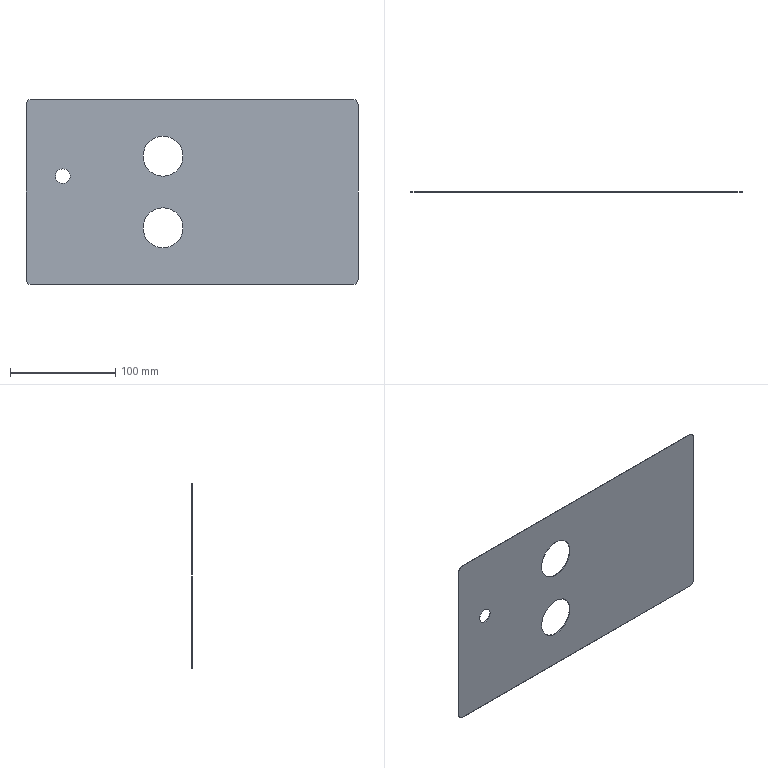Part | SolidWorks | features Extrusion 1 | 1 solid | 16 faces | box 315 x 0.6 x 176 mm | volume 31798 mm3 | cylinder 10 | plane 6 | commonest cylinder face diameters 10 x4 38 x4 14 x2
STEP:
#1=CARTESIAN_POINT('',(-95.,0.3,8.));
#2=VERTEX_POINT('',#1);
#3=CARTESIAN_POINT('',(-95.,0.3,22.));
#4=VERTEX_POINT('',#3);
#5=CARTESIAN_POINT('',(-95.,0.3,15.));
#6=DIRECTION('',(0.,1.,0.));
#7=DIRECTION('',(0.,0.,1.));
#8=AXIS2_PLACEMENT_3D('',#5,#6,#7);
#9=CIRCLE('',#8,7.);
#10=EDGE_CURVE('',#2,#4,#9,.T.);
#11=ORIENTED_EDGE('',*,*,#10,.T.);
#12=CARTESIAN_POINT('',(-95.,-0.3,22.));
#13=VERTEX_POINT('',#12);
#14=CARTESIAN_POINT('',(-95.,0.3,22.));
#15=DIRECTION('',(0.,-1.,0.));
#16=VECTOR('',#15,1000.);
#17=LINE('',#14,#16);
#18=EDGE_CURVE('',#4,#13,#17,.T.);
#19=ORIENTED_EDGE('',*,*,#18,.T.);
#20=CARTESIAN_POINT('',(-95.,-0.3,8.));
#21=VERTEX_POINT('',#20);
#22=CARTESIAN_POINT('',(-95.,-0.3,15.));
#23=DIRECTION('',(0.,1.,0.));
#24=DIRECTION('',(0.,0.,1.));
#25=AXIS2_PLACEMENT_3D('',#22,#23,#24);
#26=CIRCLE('',#25,7.);
#27=EDGE_CURVE('',#21,#13,#26,.T.);
#28=ORIENTED_EDGE('',*,*,#27,.F.);
#29=CARTESIAN_POINT('',(-95.,0.3,8.));
#30=DIRECTION('',(0.,-1.,0.));
#31=VECTOR('',#30,1000.);
#32=LINE('',#29,#31);
#33=EDGE_CURVE('',#2,#21,#32,.T.);
#34=ORIENTED_EDGE('',*,*,#33,.F.);
#35=EDGE_LOOP('',(#11,#19,#28,#34));
#36=FACE_OUTER_BOUND('',#35,.T.);
#37=CARTESIAN_POINT('',(-95.,0.3,15.));
#38=DIRECTION('',(0.,-1.,0.));
#39=DIRECTION('',(0.,0.,-1.));
#40=AXIS2_PLACEMENT_3D('',#37,#38,#39);
#41=CYLINDRICAL_SURFACE('',#40,7.);
#42=ADVANCED_FACE('',(#36),#41,.F.);
#43=CARTESIAN_POINT('',(0.,0.3,15.));
#44=VERTEX_POINT('',#43);
#45=CARTESIAN_POINT('',(0.,0.3,53.));
#46=VERTEX_POINT('',#45);
#47=CARTESIAN_POINT('',(0.,0.3,34.));
#48=DIRECTION('',(0.,1.,0.));
#49=DIRECTION('',(0.,0.,1.));
#50=AXIS2_PLACEMENT_3D('',#47,#48,#49);
#51=CIRCLE('',#50,19.);
#52=EDGE_CURVE('',#44,#46,#51,.T.);
#53=ORIENTED_EDGE('',*,*,#52,.T.);
#54=CARTESIAN_POINT('',(0.,-0.3,53.));
#55=VERTEX_POINT('',#54);
#56=CARTESIAN_POINT('',(0.,0.3,53.));
#57=DIRECTION('',(0.,-1.,0.));
#58=VECTOR('',#57,1000.);
#59=LINE('',#56,#58);
#60=EDGE_CURVE('',#46,#55,#59,.T.);
#61=ORIENTED_EDGE('',*,*,#60,.T.);
#62=CARTESIAN_POINT('',(0.,-0.3,15.));
#63=VERTEX_POINT('',#62);
#64=CARTESIAN_POINT('',(0.,-0.3,34.));
#65=DIRECTION('',(0.,1.,0.));
#66=DIRECTION('',(0.,0.,1.));
#67=AXIS2_PLACEMENT_3D('',#64,#65,#66);
#68=CIRCLE('',#67,19.);
#69=EDGE_CURVE('',#63,#55,#68,.T.);
#70=ORIENTED_EDGE('',*,*,#69,.F.);
#71=CARTESIAN_POINT('',(0.,0.3,15.));
#72=DIRECTION('',(0.,-1.,0.));
#73=VECTOR('',#72,1000.);
#74=LINE('',#71,#73);
#75=EDGE_CURVE('',#44,#63,#74,.T.);
#76=ORIENTED_EDGE('',*,*,#75,.F.);
#77=EDGE_LOOP('',(#53,#61,#70,#76));
#78=FACE_OUTER_BOUND('',#77,.T.);
#79=CARTESIAN_POINT('',(0.,0.3,34.));
#80=DIRECTION('',(0.,-1.,0.));
#81=DIRECTION('',(0.,0.,-1.));
#82=AXIS2_PLACEMENT_3D('',#79,#80,#81);
#83=CYLINDRICAL_SURFACE('',#82,19.);
#84=ADVANCED_FACE('',(#78),#83,.F.);
#85=CARTESIAN_POINT('',(0.,0.3,-53.));
#86=VERTEX_POINT('',#85);
#87=CARTESIAN_POINT('',(0.,0.3,-15.));
#88=VERTEX_POINT('',#87);
#89=CARTESIAN_POINT('',(0.,0.3,-34.));
#90=DIRECTION('',(0.,1.,0.));
#91=DIRECTION('',(0.,0.,1.));
#92=AXIS2_PLACEMENT_3D('',#89,#90,#91);
#93=CIRCLE('',#92,19.);
#94=EDGE_CURVE('',#86,#88,#93,.T.);
#95=ORIENTED_EDGE('',*,*,#94,.T.);
#96=CARTESIAN_POINT('',(0.,-0.3,-15.));
#97=VERTEX_POINT('',#96);
#98=CARTESIAN_POINT('',(0.,0.3,-15.));
#99=DIRECTION('',(0.,-1.,0.));
#100=VECTOR('',#99,1000.);
#101=LINE('',#98,#100);
#102=EDGE_CURVE('',#88,#97,#101,.T.);
#103=ORIENTED_EDGE('',*,*,#102,.T.);
#104=CARTESIAN_POINT('',(0.,-0.3,-53.));
#105=VERTEX_POINT('',#104);
#106=CARTESIAN_POINT('',(0.,-0.3,-34.));
#107=DIRECTION('',(0.,1.,0.));
#108=DIRECTION('',(0.,0.,1.));
#109=AXIS2_PLACEMENT_3D('',#106,#107,#108);
#110=CIRCLE('',#109,19.);
#111=EDGE_CURVE('',#105,#97,#110,.T.);
#112=ORIENTED_EDGE('',*,*,#111,.F.);
#113=CARTESIAN_POINT('',(0.,0.3,-53.));
#114=DIRECTION('',(0.,-1.,0.));
#115=VECTOR('',#114,1000.);
#116=LINE('',#113,#115);
#117=EDGE_CURVE('',#86,#105,#116,.T.);
#118=ORIENTED_EDGE('',*,*,#117,.F.);
#119=EDGE_LOOP('',(#95,#103,#112,#118));
#120=FACE_OUTER_BOUND('',#119,.T.);
#121=CARTESIAN_POINT('',(0.,0.3,-34.));
#122=DIRECTION('',(0.,-1.,0.));
#123=DIRECTION('',(0.,0.,-1.));
#124=AXIS2_PLACEMENT_3D('',#121,#122,#123);
#125=CYLINDRICAL_SURFACE('',#124,19.);
#126=ADVANCED_FACE('',(#120),#125,.F.);
#127=ORIENTED_EDGE('',*,*,#52,.F.);
#128=CARTESIAN_POINT('',(0.,0.3,34.));
#129=DIRECTION('',(0.,1.,0.));
#130=DIRECTION('',(0.,0.,1.));
#131=AXIS2_PLACEMENT_3D('',#128,#129,#130);
#132=CIRCLE('',#131,19.);
#133=EDGE_CURVE('',#46,#44,#132,.T.);
#134=ORIENTED_EDGE('',*,*,#133,.F.);
#135=EDGE_LOOP('',(#127,#134));
#136=FACE_BOUND('',#135,.T.);
#137=CARTESIAN_POINT('',(180.,0.3,88.));
#138=VERTEX_POINT('',#137);
#139=CARTESIAN_POINT('',(185.,0.3,83.));
#140=VERTEX_POINT('',#139);
#141=CARTESIAN_POINT('',(180.,0.3,83.));
#142=DIRECTION('',(0.,1.,0.));
#143=DIRECTION('',(0.,0.,1.));
#144=AXIS2_PLACEMENT_3D('',#141,#142,#143);
#145=CIRCLE('',#144,5.);
#146=EDGE_CURVE('',#138,#140,#145,.T.);
#147=ORIENTED_EDGE('',*,*,#146,.T.);
#148=CARTESIAN_POINT('',(185.,0.3,-83.));
#149=VERTEX_POINT('',#148);
#150=CARTESIAN_POINT('',(185.,0.3,-83.));
#151=DIRECTION('',(0.,0.,-1.));
#152=VECTOR('',#151,1000.);
#153=LINE('',#150,#152);
#154=EDGE_CURVE('',#140,#149,#153,.T.);
#155=ORIENTED_EDGE('',*,*,#154,.T.);
#156=CARTESIAN_POINT('',(180.,0.3,-88.));
#157=VERTEX_POINT('',#156);
#158=CARTESIAN_POINT('',(180.,0.3,-83.));
#159=DIRECTION('',(0.,1.,0.));
#160=DIRECTION('',(0.,0.,1.));
#161=AXIS2_PLACEMENT_3D('',#158,#159,#160);
#162=CIRCLE('',#161,5.);
#163=EDGE_CURVE('',#149,#157,#162,.T.);
#164=ORIENTED_EDGE('',*,*,#163,.T.);
#165=CARTESIAN_POINT('',(-125.,0.3,-88.));
#166=VERTEX_POINT('',#165);
#167=CARTESIAN_POINT('',(-125.,0.3,-88.));
#168=DIRECTION('',(-1.,0.,0.));
#169=VECTOR('',#168,1000.);
#170=LINE('',#167,#169);
#171=EDGE_CURVE('',#157,#166,#170,.T.);
#172=ORIENTED_EDGE('',*,*,#171,.T.);
#173=CARTESIAN_POINT('',(-130.,0.3,-83.));
#174=VERTEX_POINT('',#173);
#175=CARTESIAN_POINT('',(-125.,0.3,-83.));
#176=DIRECTION('',(0.,1.,0.));
#177=DIRECTION('',(0.,0.,1.));
#178=AXIS2_PLACEMENT_3D('',#175,#176,#177);
#179=CIRCLE('',#178,5.);
#180=EDGE_CURVE('',#166,#174,#179,.T.);
#181=ORIENTED_EDGE('',*,*,#180,.T.);
#182=CARTESIAN_POINT('',(-130.,0.3,83.));
#183=VERTEX_POINT('',#182);
#184=CARTESIAN_POINT('',(-130.,0.3,-83.));
#185=DIRECTION('',(0.,0.,1.));
#186=VECTOR('',#185,1000.);
#187=LINE('',#184,#186);
#188=EDGE_CURVE('',#174,#183,#187,.T.);
#189=ORIENTED_EDGE('',*,*,#188,.T.);
#190=CARTESIAN_POINT('',(-125.,0.3,88.));
#191=VERTEX_POINT('',#190);
#192=CARTESIAN_POINT('',(-125.,0.3,83.));
#193=DIRECTION('',(0.,1.,0.));
#194=DIRECTION('',(0.,0.,-1.));
#195=AXIS2_PLACEMENT_3D('',#192,#193,#194);
#196=CIRCLE('',#195,5.);
#197=EDGE_CURVE('',#183,#191,#196,.T.);
#198=ORIENTED_EDGE('',*,*,#197,.T.);
#199=CARTESIAN_POINT('',(-125.,0.3,88.));
#200=DIRECTION('',(1.,0.,0.));
#201=VECTOR('',#200,1000.);
#202=LINE('',#199,#201);
#203=EDGE_CURVE('',#191,#138,#202,.T.);
#204=ORIENTED_EDGE('',*,*,#203,.T.);
#205=EDGE_LOOP('',(#147,#155,#164,#172,#181,#189,#198,#204));
#206=FACE_OUTER_BOUND('',#205,.T.);
#207=ORIENTED_EDGE('',*,*,#94,.F.);
#208=CARTESIAN_POINT('',(0.,0.3,-34.));
#209=DIRECTION('',(0.,1.,0.));
#210=DIRECTION('',(0.,0.,1.));
#211=AXIS2_PLACEMENT_3D('',#208,#209,#210);
#212=CIRCLE('',#211,19.);
#213=EDGE_CURVE('',#88,#86,#212,.T.);
#214=ORIENTED_EDGE('',*,*,#213,.F.);
#215=EDGE_LOOP('',(#207,#214));
#216=FACE_BOUND('',#215,.T.);
#217=ORIENTED_EDGE('',*,*,#10,.F.);
#218=CARTESIAN_POINT('',(-95.,0.3,15.));
#219=DIRECTION('',(0.,1.,0.));
#220=DIRECTION('',(0.,0.,1.));
#221=AXIS2_PLACEMENT_3D('',#218,#219,#220);
#222=CIRCLE('',#221,7.);
#223=EDGE_CURVE('',#4,#2,#222,.T.);
#224=ORIENTED_EDGE('',*,*,#223,.F.);
#225=EDGE_LOOP('',(#217,#224));
#226=FACE_BOUND('',#225,.T.);
#227=CARTESIAN_POINT('',(180.,0.3,83.));
#228=DIRECTION('',(0.,1.,0.));
#229=DIRECTION('',(0.,0.,1.));
#230=AXIS2_PLACEMENT_3D('',#227,#228,#229);
#231=PLANE('',#230);
#232=ADVANCED_FACE('',(#136,#206,#216,#226),#231,.T.);
#233=ORIENTED_EDGE('',*,*,#69,.T.);
#234=CARTESIAN_POINT('',(0.,-0.3,34.));
#235=DIRECTION('',(0.,1.,0.));
#236=DIRECTION('',(0.,0.,1.));
#237=AXIS2_PLACEMENT_3D('',#234,#235,#236);
#238=CIRCLE('',#237,19.);
#239=EDGE_CURVE('',#55,#63,#238,.T.);
#240=ORIENTED_EDGE('',*,*,#239,.T.);
#241=EDGE_LOOP('',(#233,#240));
#242=FACE_BOUND('',#241,.T.);
#243=CARTESIAN_POINT('',(180.,-0.3,88.));
#244=VERTEX_POINT('',#243);
#245=CARTESIAN_POINT('',(185.,-0.3,83.));
#246=VERTEX_POINT('',#245);
#247=CARTESIAN_POINT('',(180.,-0.3,83.));
#248=DIRECTION('',(0.,1.,0.));
#249=DIRECTION('',(0.,0.,1.));
#250=AXIS2_PLACEMENT_3D('',#247,#248,#249);
#251=CIRCLE('',#250,5.);
#252=EDGE_CURVE('',#244,#246,#251,.T.);
#253=ORIENTED_EDGE('',*,*,#252,.F.);
#254=CARTESIAN_POINT('',(-125.,-0.3,88.));
#255=VERTEX_POINT('',#254);
#256=CARTESIAN_POINT('',(-125.,-0.3,88.));
#257=DIRECTION('',(1.,0.,0.));
#258=VECTOR('',#257,1000.);
#259=LINE('',#256,#258);
#260=EDGE_CURVE('',#255,#244,#259,.T.);
#261=ORIENTED_EDGE('',*,*,#260,.F.);
#262=CARTESIAN_POINT('',(-130.,-0.3,83.));
#263=VERTEX_POINT('',#262);
#264=CARTESIAN_POINT('',(-125.,-0.3,83.));
#265=DIRECTION('',(0.,1.,0.));
#266=DIRECTION('',(0.,0.,-1.));
#267=AXIS2_PLACEMENT_3D('',#264,#265,#266);
#268=CIRCLE('',#267,5.);
#269=EDGE_CURVE('',#263,#255,#268,.T.);
#270=ORIENTED_EDGE('',*,*,#269,.F.);
#271=CARTESIAN_POINT('',(-130.,-0.3,-83.));
#272=VERTEX_POINT('',#271);
#273=CARTESIAN_POINT('',(-130.,-0.3,-83.));
#274=DIRECTION('',(0.,0.,1.));
#275=VECTOR('',#274,1000.);
#276=LINE('',#273,#275);
#277=EDGE_CURVE('',#272,#263,#276,.T.);
#278=ORIENTED_EDGE('',*,*,#277,.F.);
#279=CARTESIAN_POINT('',(-125.,-0.3,-88.));
#280=VERTEX_POINT('',#279);
#281=CARTESIAN_POINT('',(-125.,-0.3,-83.));
#282=DIRECTION('',(0.,1.,0.));
#283=DIRECTION('',(0.,0.,1.));
#284=AXIS2_PLACEMENT_3D('',#281,#282,#283);
#285=CIRCLE('',#284,5.);
#286=EDGE_CURVE('',#280,#272,#285,.T.);
#287=ORIENTED_EDGE('',*,*,#286,.F.);
#288=CARTESIAN_POINT('',(180.,-0.3,-88.));
#289=VERTEX_POINT('',#288);
#290=CARTESIAN_POINT('',(-125.,-0.3,-88.));
#291=DIRECTION('',(-1.,0.,0.));
#292=VECTOR('',#291,1000.);
#293=LINE('',#290,#292);
#294=EDGE_CURVE('',#289,#280,#293,.T.);
#295=ORIENTED_EDGE('',*,*,#294,.F.);
#296=CARTESIAN_POINT('',(185.,-0.3,-83.));
#297=VERTEX_POINT('',#296);
#298=CARTESIAN_POINT('',(180.,-0.3,-83.));
#299=DIRECTION('',(0.,1.,0.));
#300=DIRECTION('',(0.,0.,1.));
#301=AXIS2_PLACEMENT_3D('',#298,#299,#300);
#302=CIRCLE('',#301,5.);
#303=EDGE_CURVE('',#297,#289,#302,.T.);
#304=ORIENTED_EDGE('',*,*,#303,.F.);
#305=CARTESIAN_POINT('',(185.,-0.3,-83.));
#306=DIRECTION('',(0.,0.,-1.));
#307=VECTOR('',#306,1000.);
#308=LINE('',#305,#307);
#309=EDGE_CURVE('',#246,#297,#308,.T.);
#310=ORIENTED_EDGE('',*,*,#309,.F.);
#311=EDGE_LOOP('',(#253,#261,#270,#278,#287,#295,#304,#310));
#312=FACE_OUTER_BOUND('',#311,.T.);
#313=ORIENTED_EDGE('',*,*,#111,.T.);
#314=CARTESIAN_POINT('',(0.,-0.3,-34.));
#315=DIRECTION('',(0.,1.,0.));
#316=DIRECTION('',(0.,0.,1.));
#317=AXIS2_PLACEMENT_3D('',#314,#315,#316);
#318=CIRCLE('',#317,19.);
#319=EDGE_CURVE('',#97,#105,#318,.T.);
#320=ORIENTED_EDGE('',*,*,#319,.T.);
#321=EDGE_LOOP('',(#313,#320));
#322=FACE_BOUND('',#321,.T.);
#323=ORIENTED_EDGE('',*,*,#27,.T.);
#324=CARTESIAN_POINT('',(-95.,-0.3,15.));
#325=DIRECTION('',(0.,1.,0.));
#326=DIRECTION('',(0.,0.,1.));
#327=AXIS2_PLACEMENT_3D('',#324,#325,#326);
#328=CIRCLE('',#327,7.);
#329=EDGE_CURVE('',#13,#21,#328,.T.);
#330=ORIENTED_EDGE('',*,*,#329,.T.);
#331=EDGE_LOOP('',(#323,#330));
#332=FACE_BOUND('',#331,.T.);
#333=CARTESIAN_POINT('',(180.,-0.3,83.));
#334=DIRECTION('',(0.,1.,0.));
#335=DIRECTION('',(0.,0.,1.));
#336=AXIS2_PLACEMENT_3D('',#333,#334,#335);
#337=PLANE('',#336);
#338=ADVANCED_FACE('',(#242,#312,#322,#332),#337,.F.);
#339=ORIENTED_EDGE('',*,*,#252,.T.);
#340=CARTESIAN_POINT('',(185.,0.3,83.));
#341=DIRECTION('',(0.,-1.,0.));
#342=VECTOR('',#341,1000.);
#343=LINE('',#340,#342);
#344=EDGE_CURVE('',#140,#246,#343,.T.);
#345=ORIENTED_EDGE('',*,*,#344,.F.);
#346=ORIENTED_EDGE('',*,*,#146,.F.);
#347=CARTESIAN_POINT('',(180.,0.3,88.));
#348=DIRECTION('',(0.,-1.,0.));
#349=VECTOR('',#348,1000.);
#350=LINE('',#347,#349);
#351=EDGE_CURVE('',#138,#244,#350,.T.);
#352=ORIENTED_EDGE('',*,*,#351,.T.);
#353=EDGE_LOOP('',(#339,#345,#346,#352));
#354=FACE_OUTER_BOUND('',#353,.T.);
#355=CARTESIAN_POINT('',(180.,0.3,83.));
#356=DIRECTION('',(0.,-1.,0.));
#357=DIRECTION('',(0.,0.,-1.));
#358=AXIS2_PLACEMENT_3D('',#355,#356,#357);
#359=CYLINDRICAL_SURFACE('',#358,5.);
#360=ADVANCED_FACE('',(#354),#359,.T.);
#361=ORIENTED_EDGE('',*,*,#309,.T.);
#362=CARTESIAN_POINT('',(185.,0.3,-83.));
#363=DIRECTION('',(0.,-1.,0.));
#364=VECTOR('',#363,1000.);
#365=LINE('',#362,#364);
#366=EDGE_CURVE('',#149,#297,#365,.T.);
#367=ORIENTED_EDGE('',*,*,#366,.F.);
#368=ORIENTED_EDGE('',*,*,#154,.F.);
#369=ORIENTED_EDGE('',*,*,#344,.T.);
#370=EDGE_LOOP('',(#361,#367,#368,#369));
#371=FACE_OUTER_BOUND('',#370,.T.);
#372=CARTESIAN_POINT('',(185.,0.3,-83.));
#373=DIRECTION('',(-1.,0.,0.));
#374=DIRECTION('',(0.,0.,1.));
#375=AXIS2_PLACEMENT_3D('',#372,#373,#374);
#376=PLANE('',#375);
#377=ADVANCED_FACE('',(#371),#376,.F.);
#378=ORIENTED_EDGE('',*,*,#303,.T.);
#379=CARTESIAN_POINT('',(180.,0.3,-88.));
#380=DIRECTION('',(0.,-1.,0.));
#381=VECTOR('',#380,1000.);
#382=LINE('',#379,#381);
#383=EDGE_CURVE('',#157,#289,#382,.T.);
#384=ORIENTED_EDGE('',*,*,#383,.F.);
#385=ORIENTED_EDGE('',*,*,#163,.F.);
#386=ORIENTED_EDGE('',*,*,#366,.T.);
#387=EDGE_LOOP('',(#378,#384,#385,#386));
#388=FACE_OUTER_BOUND('',#387,.T.);
#389=CARTESIAN_POINT('',(180.,0.3,-83.));
#390=DIRECTION('',(0.,-1.,0.));
#391=DIRECTION('',(0.,0.,-1.));
#392=AXIS2_PLACEMENT_3D('',#389,#390,#391);
#393=CYLINDRICAL_SURFACE('',#392,5.);
#394=ADVANCED_FACE('',(#388),#393,.T.);
#395=ORIENTED_EDGE('',*,*,#294,.T.);
#396=CARTESIAN_POINT('',(-125.,0.3,-88.));
#397=DIRECTION('',(0.,-1.,0.));
#398=VECTOR('',#397,1000.);
#399=LINE('',#396,#398);
#400=EDGE_CURVE('',#166,#280,#399,.T.);
#401=ORIENTED_EDGE('',*,*,#400,.F.);
#402=ORIENTED_EDGE('',*,*,#171,.F.);
#403=ORIENTED_EDGE('',*,*,#383,.T.);
#404=EDGE_LOOP('',(#395,#401,#402,#403));
#405=FACE_OUTER_BOUND('',#404,.T.);
#406=CARTESIAN_POINT('',(-125.,0.3,-88.));
#407=DIRECTION('',(0.,0.,1.));
#408=DIRECTION('',(1.,0.,0.));
#409=AXIS2_PLACEMENT_3D('',#406,#407,#408);
#410=PLANE('',#409);
#411=ADVANCED_FACE('',(#405),#410,.F.);
#412=ORIENTED_EDGE('',*,*,#286,.T.);
#413=CARTESIAN_POINT('',(-130.,0.3,-83.));
#414=DIRECTION('',(0.,-1.,0.));
#415=VECTOR('',#414,1000.);
#416=LINE('',#413,#415);
#417=EDGE_CURVE('',#174,#272,#416,.T.);
#418=ORIENTED_EDGE('',*,*,#417,.F.);
#419=ORIENTED_EDGE('',*,*,#180,.F.);
#420=ORIENTED_EDGE('',*,*,#400,.T.);
#421=EDGE_LOOP('',(#412,#418,#419,#420));
#422=FACE_OUTER_BOUND('',#421,.T.);
#423=CARTESIAN_POINT('',(-125.,0.3,-83.));
#424=DIRECTION('',(0.,-1.,0.));
#425=DIRECTION('',(0.,0.,-1.));
#426=AXIS2_PLACEMENT_3D('',#423,#424,#425);
#427=CYLINDRICAL_SURFACE('',#426,5.);
#428=ADVANCED_FACE('',(#422),#427,.T.);
#429=ORIENTED_EDGE('',*,*,#277,.T.);
#430=CARTESIAN_POINT('',(-130.,0.3,83.));
#431=DIRECTION('',(0.,-1.,0.));
#432=VECTOR('',#431,1000.);
#433=LINE('',#430,#432);
#434=EDGE_CURVE('',#183,#263,#433,.T.);
#435=ORIENTED_EDGE('',*,*,#434,.F.);
#436=ORIENTED_EDGE('',*,*,#188,.F.);
#437=ORIENTED_EDGE('',*,*,#417,.T.);
#438=EDGE_LOOP('',(#429,#435,#436,#437));
#439=FACE_OUTER_BOUND('',#438,.T.);
#440=CARTESIAN_POINT('',(-130.,0.3,-83.));
#441=DIRECTION('',(1.,0.,0.));
#442=DIRECTION('',(0.,0.,-1.));
#443=AXIS2_PLACEMENT_3D('',#440,#441,#442);
#444=PLANE('',#443);
#445=ADVANCED_FACE('',(#439),#444,.F.);
#446=ORIENTED_EDGE('',*,*,#269,.T.);
#447=CARTESIAN_POINT('',(-125.,0.3,88.));
#448=DIRECTION('',(0.,-1.,0.));
#449=VECTOR('',#448,1000.);
#450=LINE('',#447,#449);
#451=EDGE_CURVE('',#191,#255,#450,.T.);
#452=ORIENTED_EDGE('',*,*,#451,.F.);
#453=ORIENTED_EDGE('',*,*,#197,.F.);
#454=ORIENTED_EDGE('',*,*,#434,.T.);
#455=EDGE_LOOP('',(#446,#452,#453,#454));
#456=FACE_OUTER_BOUND('',#455,.T.);
#457=CARTESIAN_POINT('',(-125.,0.3,83.));
#458=DIRECTION('',(0.,-1.,0.));
#459=DIRECTION('',(0.,0.,-1.));
#460=AXIS2_PLACEMENT_3D('',#457,#458,#459);
#461=CYLINDRICAL_SURFACE('',#460,5.);
#462=ADVANCED_FACE('',(#456),#461,.T.);
#463=ORIENTED_EDGE('',*,*,#260,.T.);
#464=ORIENTED_EDGE('',*,*,#351,.F.);
#465=ORIENTED_EDGE('',*,*,#203,.F.);
#466=ORIENTED_EDGE('',*,*,#451,.T.);
#467=EDGE_LOOP('',(#463,#464,#465,#466));
#468=FACE_OUTER_BOUND('',#467,.T.);
#469=CARTESIAN_POINT('',(-125.,0.3,88.));
#470=DIRECTION('',(0.,0.,-1.));
#471=DIRECTION('',(-1.,0.,0.));
#472=AXIS2_PLACEMENT_3D('',#469,#470,#471);
#473=PLANE('',#472);
#474=ADVANCED_FACE('',(#468),#473,.F.);
#475=ORIENTED_EDGE('',*,*,#102,.F.);
#476=ORIENTED_EDGE('',*,*,#213,.T.);
#477=ORIENTED_EDGE('',*,*,#117,.T.);
#478=ORIENTED_EDGE('',*,*,#319,.F.);
#479=EDGE_LOOP('',(#475,#476,#477,#478));
#480=FACE_OUTER_BOUND('',#479,.T.);
#481=CARTESIAN_POINT('',(0.,0.3,-34.));
#482=DIRECTION('',(0.,-1.,0.));
#483=DIRECTION('',(0.,0.,-1.));
#484=AXIS2_PLACEMENT_3D('',#481,#482,#483);
#485=CYLINDRICAL_SURFACE('',#484,19.);
#486=ADVANCED_FACE('',(#480),#485,.F.);
#487=ORIENTED_EDGE('',*,*,#60,.F.);
#488=ORIENTED_EDGE('',*,*,#133,.T.);
#489=ORIENTED_EDGE('',*,*,#75,.T.);
#490=ORIENTED_EDGE('',*,*,#239,.F.);
#491=EDGE_LOOP('',(#487,#488,#489,#490));
#492=FACE_OUTER_BOUND('',#491,.T.);
#493=CARTESIAN_POINT('',(0.,0.3,34.));
#494=DIRECTION('',(0.,-1.,0.));
#495=DIRECTION('',(0.,0.,-1.));
#496=AXIS2_PLACEMENT_3D('',#493,#494,#495);
#497=CYLINDRICAL_SURFACE('',#496,19.);
#498=ADVANCED_FACE('',(#492),#497,.F.);
#499=ORIENTED_EDGE('',*,*,#18,.F.);
#500=ORIENTED_EDGE('',*,*,#223,.T.);
#501=ORIENTED_EDGE('',*,*,#33,.T.);
#502=ORIENTED_EDGE('',*,*,#329,.F.);
#503=EDGE_LOOP('',(#499,#500,#501,#502));
#504=FACE_OUTER_BOUND('',#503,.T.);
#505=CARTESIAN_POINT('',(-95.,0.3,15.));
#506=DIRECTION('',(0.,-1.,0.));
#507=DIRECTION('',(0.,0.,-1.));
#508=AXIS2_PLACEMENT_3D('',#505,#506,#507);
#509=CYLINDRICAL_SURFACE('',#508,7.);
#510=ADVANCED_FACE('',(#504),#509,.F.);
#511=CLOSED_SHELL('',(#42,#84,#126,#232,#338,#360,#377,#394,#411,#428,#445,#462,#474,#486,#498,#510));
#512=MANIFOLD_SOLID_BREP('',#511);
#513=CARTESIAN_POINT('',(0.,0.,0.));
#514=DIRECTION('',(0.,0.,1.));
#515=DIRECTION('',(1.,0.,0.));
#516=AXIS2_PLACEMENT_3D('',#513,#514,#515);
#517=(LENGTH_UNIT()NAMED_UNIT(*)SI_UNIT(.MILLI.,.METRE.));
#518=UNCERTAINTY_MEASURE_WITH_UNIT(LENGTH_MEASURE(0.00001),#517,'','');
#519=(NAMED_UNIT(*)PLANE_ANGLE_UNIT()SI_UNIT($,.RADIAN.));
#520=(NAMED_UNIT(*)SI_UNIT($,.STERADIAN.)SOLID_ANGLE_UNIT());
#521=(GEOMETRIC_REPRESENTATION_CONTEXT(3)GLOBAL_UNCERTAINTY_ASSIGNED_CONTEXT((#518))GLOBAL_UNIT_ASSIGNED_CONTEXT((#517,#519,#520))REPRESENTATION_CONTEXT('',''));
#522=ADVANCED_BREP_SHAPE_REPRESENTATION('',(#512,#516),#521);